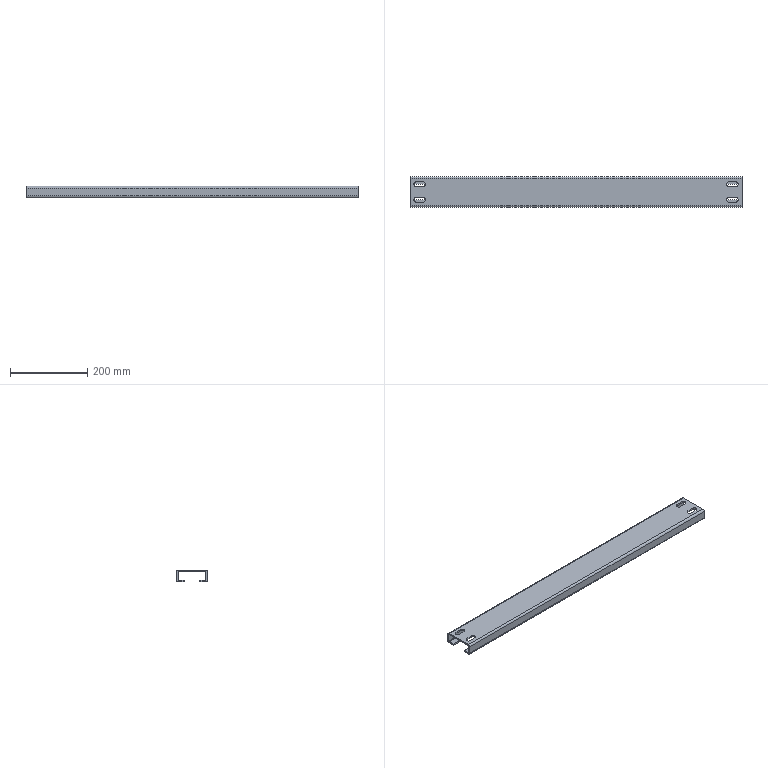Part | 1 solid | 58 faces | box 860 x 80 x 30 mm | volume 540783 mm3 | plane 38 | cylinder 20 | commonest cylinder face diameters 13 x12 2 x4 10 x4